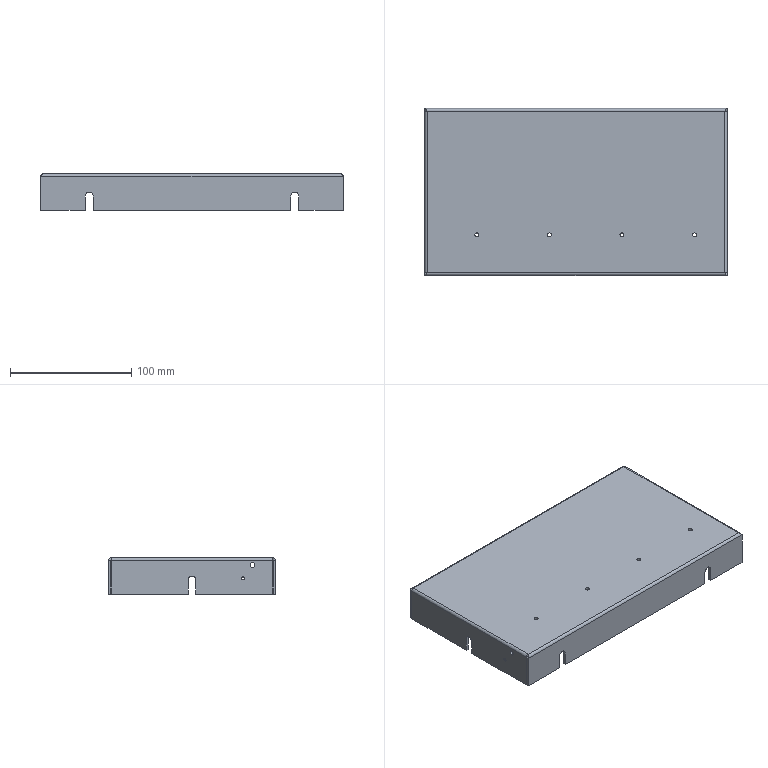Part | STEP file | 1 solid | 82 faces | box 250 x 138 x 30 mm | volume 110009 mm3 | plane 44 | cylinder 34 | spline 4 | commonest cylinder face diameters 3.3 x8 6.6 x8 0.2 x4 2.5 x4 4 x4 4.2 x4